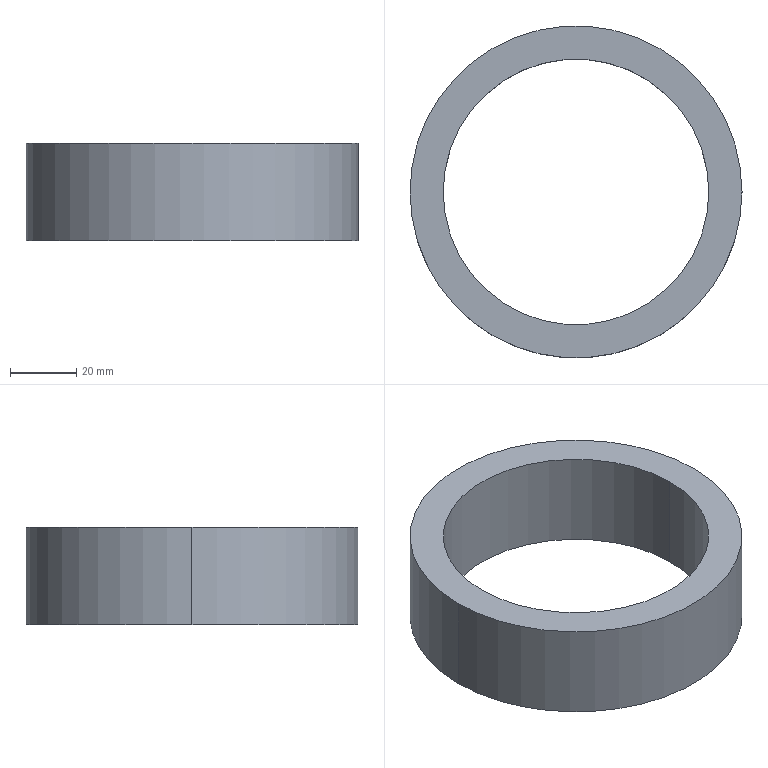Part | SolidWorks | features Extrusion 1 | 1 solid | 6 faces | box 100 x 100 x 29.5 mm | volume 83409 mm3 | cylinder 4 | plane 2 | commonest cylinder face diameters 80 x2 100 x2
STEP:
#1=CARTESIAN_POINT('',(-40.,0.,29.5));
#2=VERTEX_POINT('',#1);
#3=CARTESIAN_POINT('',(40.,0.,29.5));
#4=VERTEX_POINT('',#3);
#5=CARTESIAN_POINT('',(0.,0.,29.5));
#6=DIRECTION('',(0.,0.,1.));
#7=DIRECTION('',(1.,0.,0.));
#8=AXIS2_PLACEMENT_3D('',#5,#6,#7);
#9=CIRCLE('',#8,40.);
#10=EDGE_CURVE('',#2,#4,#9,.T.);
#11=ORIENTED_EDGE('',*,*,#10,.T.);
#12=CARTESIAN_POINT('',(40.,0.,0.));
#13=VERTEX_POINT('',#12);
#14=CARTESIAN_POINT('',(40.,0.,29.5));
#15=DIRECTION('',(0.,0.,-1.));
#16=VECTOR('',#15,1000.);
#17=LINE('',#14,#16);
#18=EDGE_CURVE('',#4,#13,#17,.T.);
#19=ORIENTED_EDGE('',*,*,#18,.T.);
#20=CARTESIAN_POINT('',(-40.,0.,0.));
#21=VERTEX_POINT('',#20);
#22=CARTESIAN_POINT('',(0.,0.,0.));
#23=DIRECTION('',(0.,0.,1.));
#24=DIRECTION('',(1.,0.,0.));
#25=AXIS2_PLACEMENT_3D('',#22,#23,#24);
#26=CIRCLE('',#25,40.);
#27=EDGE_CURVE('',#21,#13,#26,.T.);
#28=ORIENTED_EDGE('',*,*,#27,.F.);
#29=CARTESIAN_POINT('',(-40.,0.,29.5));
#30=DIRECTION('',(0.,0.,-1.));
#31=VECTOR('',#30,1000.);
#32=LINE('',#29,#31);
#33=EDGE_CURVE('',#2,#21,#32,.T.);
#34=ORIENTED_EDGE('',*,*,#33,.F.);
#35=EDGE_LOOP('',(#11,#19,#28,#34));
#36=FACE_OUTER_BOUND('',#35,.T.);
#37=CARTESIAN_POINT('',(0.,0.,29.5));
#38=DIRECTION('',(0.,0.,-1.));
#39=DIRECTION('',(-1.,0.,0.));
#40=AXIS2_PLACEMENT_3D('',#37,#38,#39);
#41=CYLINDRICAL_SURFACE('',#40,40.);
#42=ADVANCED_FACE('',(#36),#41,.F.);
#43=CARTESIAN_POINT('',(50.,0.,29.5));
#44=VERTEX_POINT('',#43);
#45=CARTESIAN_POINT('',(-50.,0.,29.5));
#46=VERTEX_POINT('',#45);
#47=CARTESIAN_POINT('',(0.,0.,29.5));
#48=DIRECTION('',(0.,0.,1.));
#49=DIRECTION('',(1.,0.,0.));
#50=AXIS2_PLACEMENT_3D('',#47,#48,#49);
#51=CIRCLE('',#50,50.);
#52=EDGE_CURVE('',#44,#46,#51,.T.);
#53=ORIENTED_EDGE('',*,*,#52,.F.);
#54=CARTESIAN_POINT('',(50.,0.,0.));
#55=VERTEX_POINT('',#54);
#56=CARTESIAN_POINT('',(50.,0.,29.5));
#57=DIRECTION('',(0.,0.,-1.));
#58=VECTOR('',#57,1000.);
#59=LINE('',#56,#58);
#60=EDGE_CURVE('',#44,#55,#59,.T.);
#61=ORIENTED_EDGE('',*,*,#60,.T.);
#62=CARTESIAN_POINT('',(-50.,0.,0.));
#63=VERTEX_POINT('',#62);
#64=CARTESIAN_POINT('',(0.,0.,0.));
#65=DIRECTION('',(0.,0.,1.));
#66=DIRECTION('',(1.,0.,0.));
#67=AXIS2_PLACEMENT_3D('',#64,#65,#66);
#68=CIRCLE('',#67,50.);
#69=EDGE_CURVE('',#55,#63,#68,.T.);
#70=ORIENTED_EDGE('',*,*,#69,.T.);
#71=CARTESIAN_POINT('',(-50.,0.,29.5));
#72=DIRECTION('',(0.,0.,-1.));
#73=VECTOR('',#72,1000.);
#74=LINE('',#71,#73);
#75=EDGE_CURVE('',#46,#63,#74,.T.);
#76=ORIENTED_EDGE('',*,*,#75,.F.);
#77=EDGE_LOOP('',(#53,#61,#70,#76));
#78=FACE_OUTER_BOUND('',#77,.T.);
#79=CARTESIAN_POINT('',(0.,0.,29.5));
#80=DIRECTION('',(0.,0.,-1.));
#81=DIRECTION('',(-1.,0.,0.));
#82=AXIS2_PLACEMENT_3D('',#79,#80,#81);
#83=CYLINDRICAL_SURFACE('',#82,50.);
#84=ADVANCED_FACE('',(#78),#83,.T.);
#85=CARTESIAN_POINT('',(0.,0.,29.5));
#86=DIRECTION('',(0.,0.,1.));
#87=DIRECTION('',(1.,0.,0.));
#88=AXIS2_PLACEMENT_3D('',#85,#86,#87);
#89=CIRCLE('',#88,50.);
#90=EDGE_CURVE('',#46,#44,#89,.T.);
#91=ORIENTED_EDGE('',*,*,#90,.T.);
#92=ORIENTED_EDGE('',*,*,#52,.T.);
#93=EDGE_LOOP('',(#91,#92));
#94=FACE_OUTER_BOUND('',#93,.T.);
#95=ORIENTED_EDGE('',*,*,#10,.F.);
#96=CARTESIAN_POINT('',(0.,0.,29.5));
#97=DIRECTION('',(0.,0.,1.));
#98=DIRECTION('',(1.,0.,0.));
#99=AXIS2_PLACEMENT_3D('',#96,#97,#98);
#100=CIRCLE('',#99,40.);
#101=EDGE_CURVE('',#4,#2,#100,.T.);
#102=ORIENTED_EDGE('',*,*,#101,.F.);
#103=EDGE_LOOP('',(#95,#102));
#104=FACE_BOUND('',#103,.T.);
#105=CARTESIAN_POINT('',(0.,0.,29.5));
#106=DIRECTION('',(0.,0.,1.));
#107=DIRECTION('',(1.,0.,0.));
#108=AXIS2_PLACEMENT_3D('',#105,#106,#107);
#109=PLANE('',#108);
#110=ADVANCED_FACE('',(#94,#104),#109,.T.);
#111=CARTESIAN_POINT('',(0.,0.,0.));
#112=DIRECTION('',(0.,0.,1.));
#113=DIRECTION('',(1.,0.,0.));
#114=AXIS2_PLACEMENT_3D('',#111,#112,#113);
#115=CIRCLE('',#114,50.);
#116=EDGE_CURVE('',#63,#55,#115,.T.);
#117=ORIENTED_EDGE('',*,*,#116,.F.);
#118=ORIENTED_EDGE('',*,*,#69,.F.);
#119=EDGE_LOOP('',(#117,#118));
#120=FACE_OUTER_BOUND('',#119,.T.);
#121=ORIENTED_EDGE('',*,*,#27,.T.);
#122=CARTESIAN_POINT('',(0.,0.,0.));
#123=DIRECTION('',(0.,0.,1.));
#124=DIRECTION('',(1.,0.,0.));
#125=AXIS2_PLACEMENT_3D('',#122,#123,#124);
#126=CIRCLE('',#125,40.);
#127=EDGE_CURVE('',#13,#21,#126,.T.);
#128=ORIENTED_EDGE('',*,*,#127,.T.);
#129=EDGE_LOOP('',(#121,#128));
#130=FACE_BOUND('',#129,.T.);
#131=CARTESIAN_POINT('',(0.,0.,0.));
#132=DIRECTION('',(0.,0.,1.));
#133=DIRECTION('',(1.,0.,0.));
#134=AXIS2_PLACEMENT_3D('',#131,#132,#133);
#135=PLANE('',#134);
#136=ADVANCED_FACE('',(#120,#130),#135,.F.);
#137=ORIENTED_EDGE('',*,*,#60,.F.);
#138=ORIENTED_EDGE('',*,*,#90,.F.);
#139=ORIENTED_EDGE('',*,*,#75,.T.);
#140=ORIENTED_EDGE('',*,*,#116,.T.);
#141=EDGE_LOOP('',(#137,#138,#139,#140));
#142=FACE_OUTER_BOUND('',#141,.T.);
#143=CARTESIAN_POINT('',(0.,0.,29.5));
#144=DIRECTION('',(0.,0.,-1.));
#145=DIRECTION('',(-1.,0.,0.));
#146=AXIS2_PLACEMENT_3D('',#143,#144,#145);
#147=CYLINDRICAL_SURFACE('',#146,50.);
#148=ADVANCED_FACE('',(#142),#147,.T.);
#149=ORIENTED_EDGE('',*,*,#18,.F.);
#150=ORIENTED_EDGE('',*,*,#101,.T.);
#151=ORIENTED_EDGE('',*,*,#33,.T.);
#152=ORIENTED_EDGE('',*,*,#127,.F.);
#153=EDGE_LOOP('',(#149,#150,#151,#152));
#154=FACE_OUTER_BOUND('',#153,.T.);
#155=CARTESIAN_POINT('',(0.,0.,29.5));
#156=DIRECTION('',(0.,0.,-1.));
#157=DIRECTION('',(-1.,0.,0.));
#158=AXIS2_PLACEMENT_3D('',#155,#156,#157);
#159=CYLINDRICAL_SURFACE('',#158,40.);
#160=ADVANCED_FACE('',(#154),#159,.F.);
#161=CLOSED_SHELL('',(#42,#84,#110,#136,#148,#160));
#162=MANIFOLD_SOLID_BREP('',#161);
#163=CARTESIAN_POINT('',(0.,0.,0.));
#164=DIRECTION('',(0.,0.,1.));
#165=DIRECTION('',(1.,0.,0.));
#166=AXIS2_PLACEMENT_3D('',#163,#164,#165);
#167=(LENGTH_UNIT()NAMED_UNIT(*)SI_UNIT(.MILLI.,.METRE.));
#168=UNCERTAINTY_MEASURE_WITH_UNIT(LENGTH_MEASURE(0.00001),#167,'','');
#169=(NAMED_UNIT(*)PLANE_ANGLE_UNIT()SI_UNIT($,.RADIAN.));
#170=(NAMED_UNIT(*)SI_UNIT($,.STERADIAN.)SOLID_ANGLE_UNIT());
#171=(GEOMETRIC_REPRESENTATION_CONTEXT(3)GLOBAL_UNCERTAINTY_ASSIGNED_CONTEXT((#168))GLOBAL_UNIT_ASSIGNED_CONTEXT((#167,#169,#170))REPRESENTATION_CONTEXT('',''));
#172=ADVANCED_BREP_SHAPE_REPRESENTATION('',(#162,#166),#171);